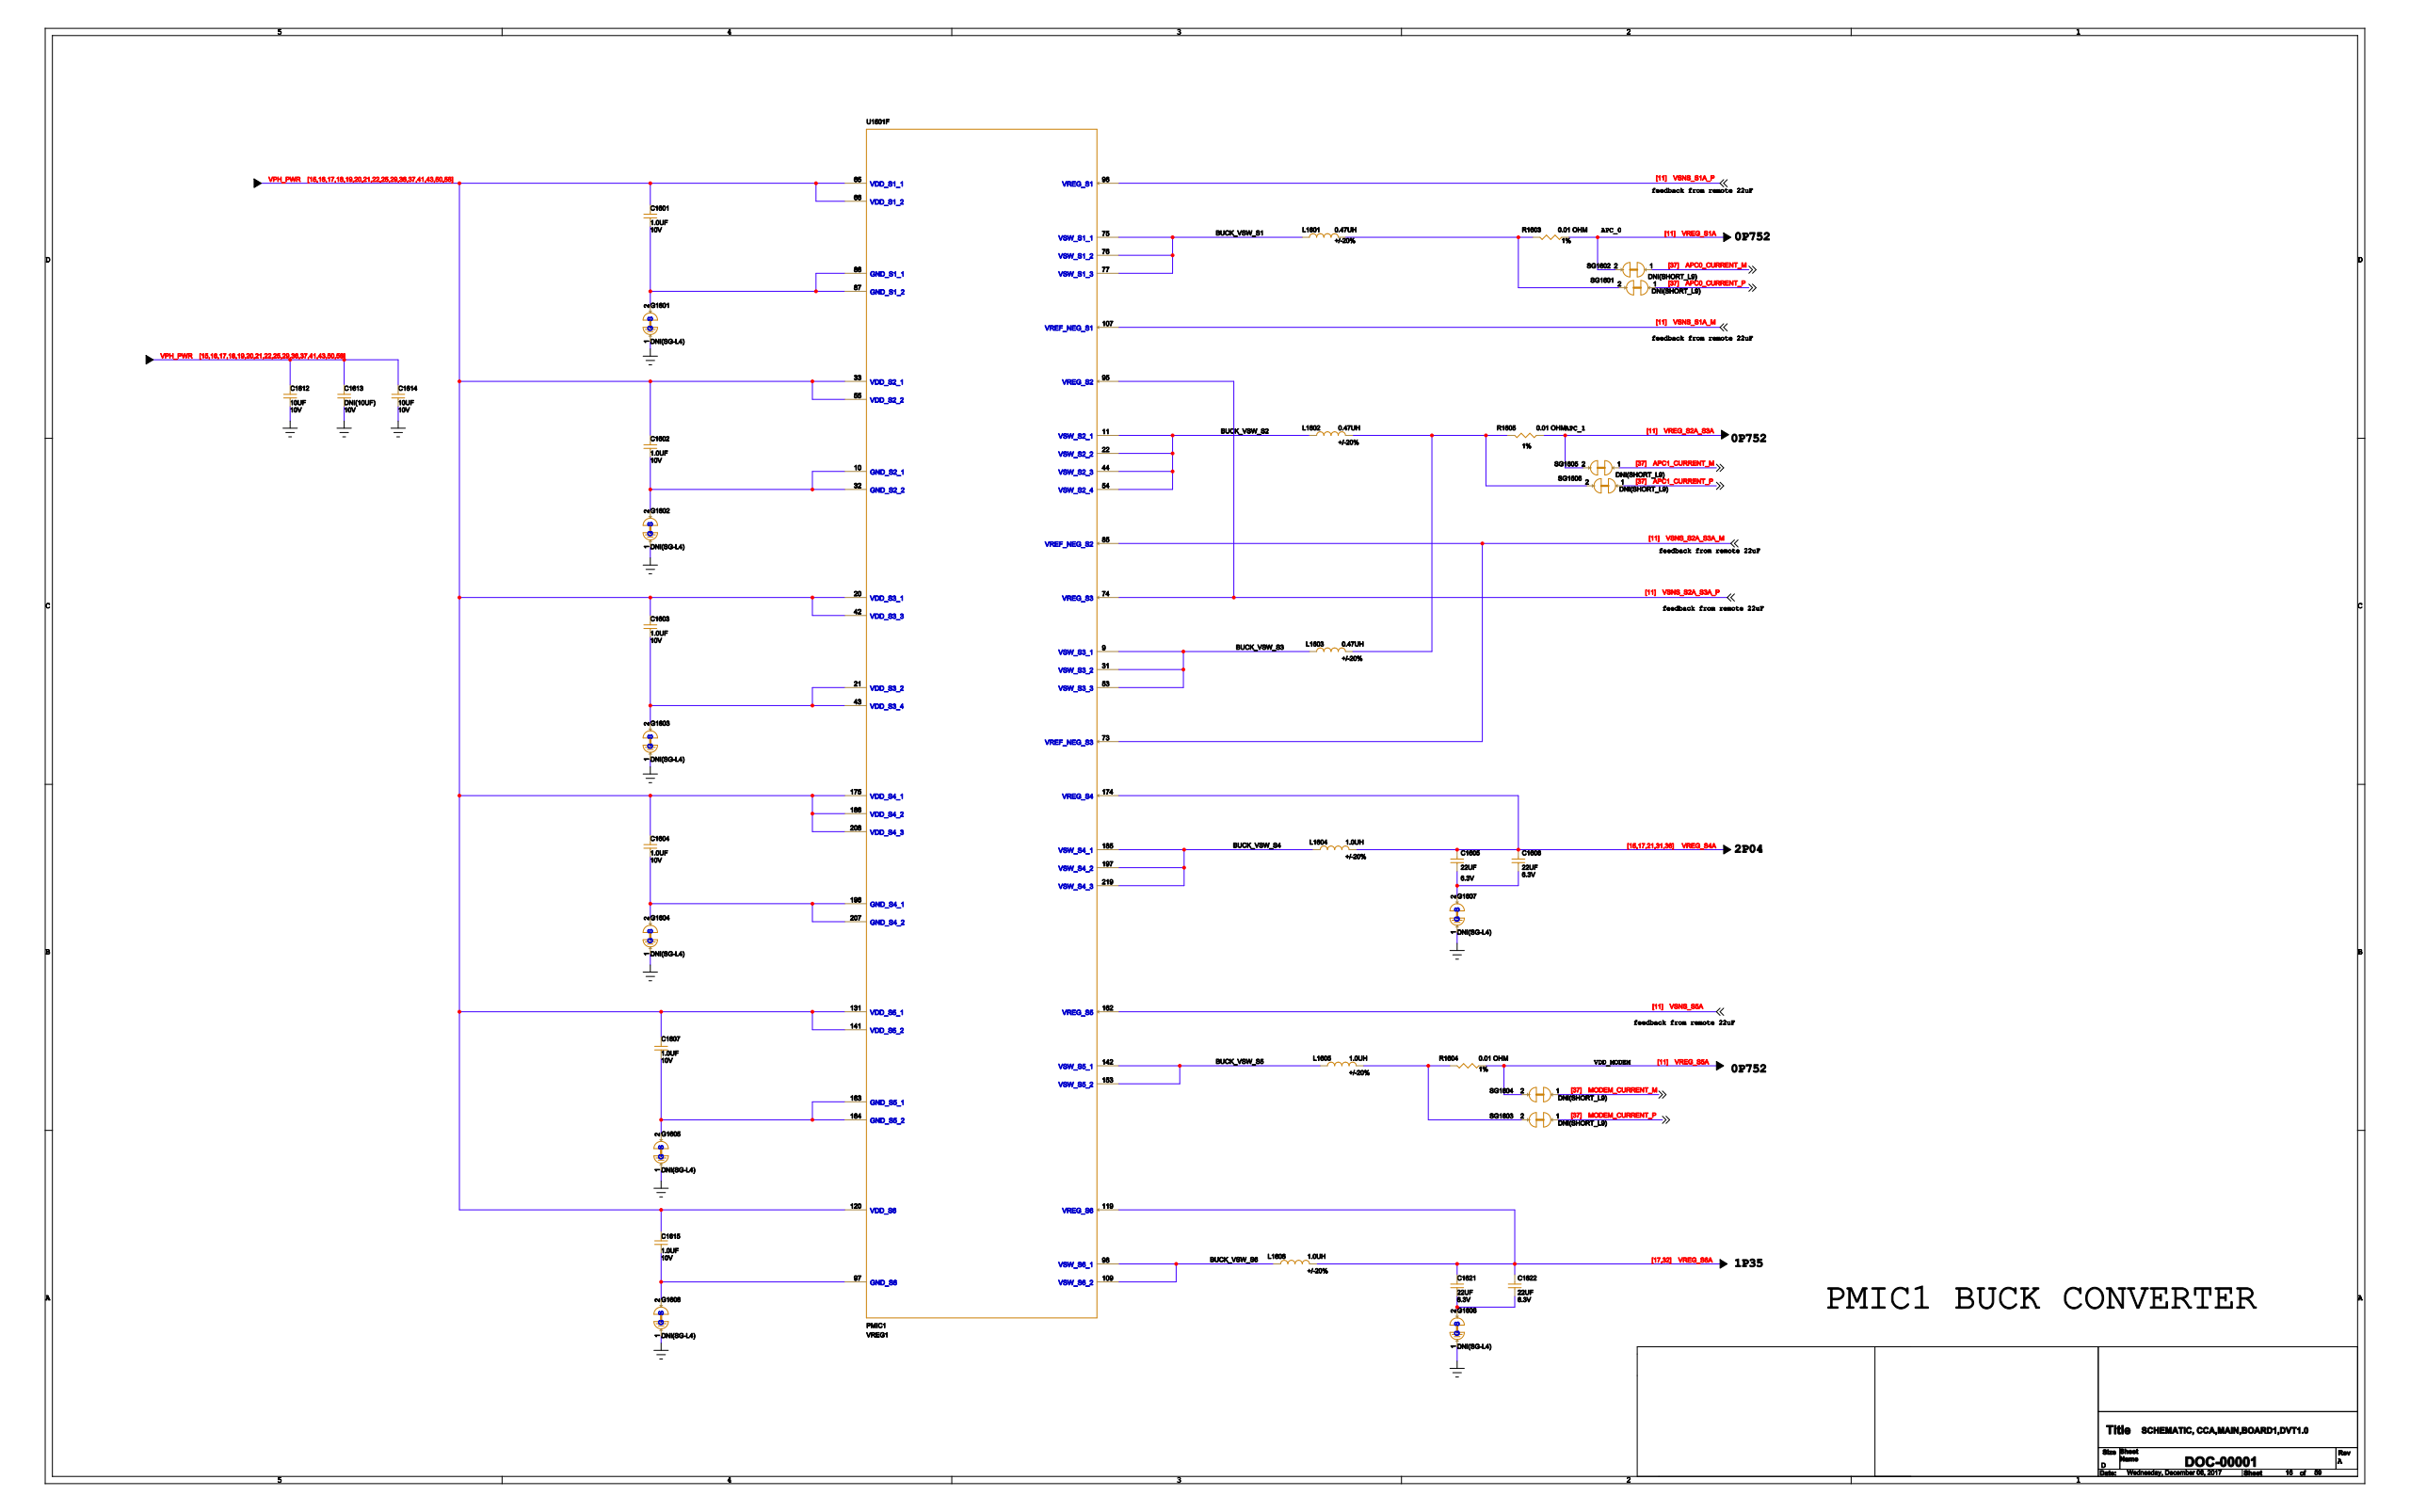Circuit board | KiCad | 1657 parts | 1365 nets | one sheet of the schematic
Parts on this sheet (reference | value | footprint):
C1601
C1602
C1603
C1604
C1605
C1606
C1607
C1612
C1613
C1614
C1615
C1621
C1622
G1601
G1602
G1603
G1604
G1605
G1606
G1607
G1608
L1601
L1602
L1603
L1604
L1605
L1606
R1603
R1604
R1605
SG1601
SG1602
SG1603
SG1604
SG1605
SG1606
U1501
Nets of these parts (net: part-pin ...):
GND: C1612-1 C1613-1 C1614-1 G1601-1 G1602-1 G1603-1 G1604-1 G1605-1 G1606-1 G1607-1 G1608-1
VPH_PWR: C1601-2 C1602-2 C1603-2 C1604-2 C1607-2 C1612-2 C1613-2 C1614-2 C1615-2 U1501-3 U1501-20 U1501-25 U1501-33 U1501-37 U1501-42 U1501-55 U1501-65 U1501-66 U1501-120 U1501-131 U1501-141 U1501-175 U1501-186 U1501-208
APC0_CURRENT_P: SG1601-1
N17088011: L1601-2 R1603-1 SG1601-2
N17087224: C1605-1 C1606-1 G1607-2
VREG_S6A: C1621-2 C1622-2 L1606-2 U1501-119
N17087286: C1601-1 G1601-2 U1501-86 U1501-87
ODEM_CURRENT_P: SG1603-1
N17087276: L1605-2 R1604-1 SG1603-2
APC0_CURRENT_M: SG1602-1
VREG_S1A: R1603-2 SG1602-2
APC1_CURRENT_M: SG1605-1
VREG_S2A_S3A: R1605-2 SG1605-2
VREG_S4A: C1605-2 C1606-2 L1604-2 U1501-174
VREG_S5A: R1604-2 SG1604-2
VSNS_S5A: U1501-162
VSNS_S2A_S3A_M: U1501-73 U1501-85
N17087178: C1615-1 G1606-2 U1501-97
APC1_CURRENT_P: SG1606-1
N17087252: L1602-2 L1603-2 R1605-1 SG1606-2
VSNS_S2A_S3A_P: U1501-74 U1501-95
ODEM_CURRENT_M: SG1604-1
N17087328: C1604-1 G1604-2 U1501-196 U1501-207
N17087318: C1603-1 G1603-2 U1501-21 U1501-43
VSNS_S1A_M: U1501-107
VSNS_S1A_P: U1501-96
N17087344: C1607-1 G1605-2 U1501-163 U1501-164
N17087300: C1602-1 G1602-2 U1501-10 U1501-32
N20468977: C1621-1 C1622-1 G1608-2
BUCK_VSW_S1: L1601-1 U1501-75 U1501-76 U1501-77
BUCK_VSW_S4: L1604-1 U1501-185 U1501-197 U1501-219
BUCK_VSW_S5: L1605-1 U1501-142 U1501-153
BUCK_VSW_S3: L1603-1 U1501-9 U1501-31 U1501-53
BUCK_VSW_S6: L1606-1 U1501-98 U1501-109
BUCK_VSW_S2: L1602-1 U1501-11 U1501-22 U1501-44 U1501-54